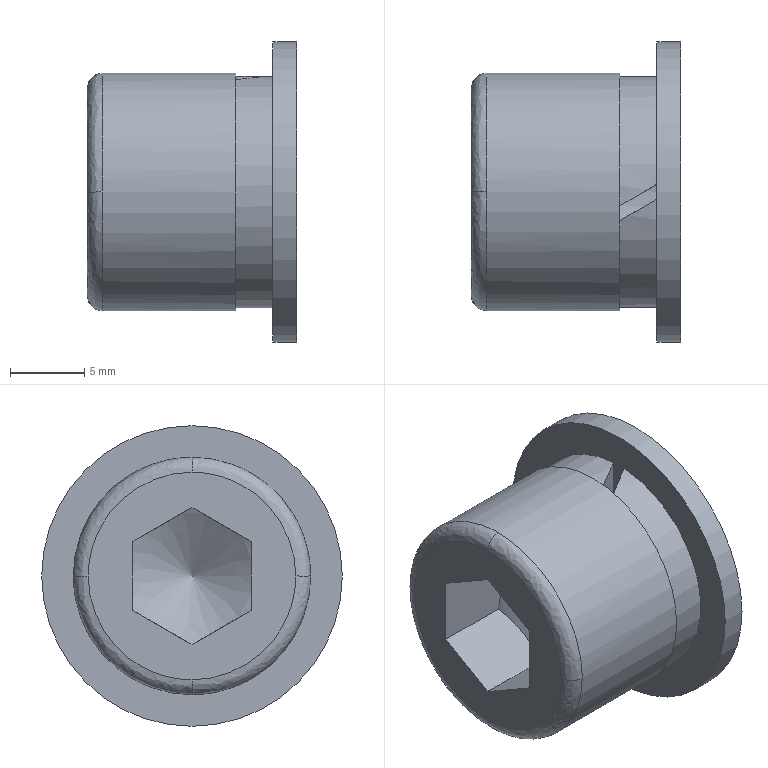Part | NX | features BREP 2 | 2 solids | 23 faces | box 14.1 x 20.25 x 20.25 mm | volume 2295 mm3 | plane 13 | cylinder 5 | spline 4 | cone 1 | commonest cylinder face diameters 10.2 x1 10.7 x1 15.6 x1 16 x1 20.25 x1
STEP:
#1=CARTESIAN_POINT('',(408.903,695.69,-5.1));
#2=VERTEX_POINT('',#1);
#3=CARTESIAN_POINT('',(408.903,695.69,0.));
#4=DIRECTION('',(1.,0.,0.));
#5=DIRECTION('',(0.,0.,-1.));
#6=AXIS2_PLACEMENT_3D('',#3,#4,#5);
#7=CIRCLE('',#6,5.1);
#8=EDGE_CURVE('',#2,#2,#7,.T.);
#9=ORIENTED_EDGE('',*,*,#8,.T.);
#10=EDGE_LOOP('',(#9));
#11=FACE_BOUND('',#10,.T.);
#12=CARTESIAN_POINT('',(408.903,695.69,-10.125));
#13=VERTEX_POINT('',#12);
#14=CARTESIAN_POINT('',(408.903,695.69,0.));
#15=DIRECTION('',(1.,0.,0.));
#16=DIRECTION('',(0.,0.,-1.));
#17=AXIS2_PLACEMENT_3D('',#14,#15,#16);
#18=CIRCLE('',#17,10.125);
#19=EDGE_CURVE('',#13,#13,#18,.T.);
#20=ORIENTED_EDGE('',*,*,#19,.F.);
#21=EDGE_LOOP('',(#20));
#22=FACE_BOUND('',#21,.T.);
#23=CARTESIAN_POINT('',(408.903,705.815,0.));
#24=DIRECTION('',(1.,0.,0.));
#25=DIRECTION('',(0.,0.,1.));
#26=AXIS2_PLACEMENT_3D('',#23,#24,#25);
#27=PLANE('',#26);
#28=ADVANCED_FACE('',(#11,#22),#27,.F.);
#29=CARTESIAN_POINT('',(410.503,695.69,-5.1));
#30=VERTEX_POINT('',#29);
#31=CARTESIAN_POINT('',(410.503,695.69,0.));
#32=DIRECTION('',(1.,0.,0.));
#33=DIRECTION('',(0.,0.,-1.));
#34=AXIS2_PLACEMENT_3D('',#31,#32,#33);
#35=CIRCLE('',#34,5.1);
#36=EDGE_CURVE('',#30,#30,#35,.T.);
#37=ORIENTED_EDGE('',*,*,#36,.F.);
#38=EDGE_LOOP('',(#37));
#39=FACE_BOUND('',#38,.T.);
#40=CARTESIAN_POINT('',(410.503,695.69,-10.125));
#41=VERTEX_POINT('',#40);
#42=CARTESIAN_POINT('',(410.503,695.69,0.));
#43=DIRECTION('',(1.,0.,0.));
#44=DIRECTION('',(0.,0.,-1.));
#45=AXIS2_PLACEMENT_3D('',#42,#43,#44);
#46=CIRCLE('',#45,10.125);
#47=EDGE_CURVE('',#41,#41,#46,.T.);
#48=ORIENTED_EDGE('',*,*,#47,.T.);
#49=EDGE_LOOP('',(#48));
#50=FACE_BOUND('',#49,.T.);
#51=CARTESIAN_POINT('',(410.503,700.79,0.));
#52=DIRECTION('',(1.,0.,0.));
#53=DIRECTION('',(0.,0.,1.));
#54=AXIS2_PLACEMENT_3D('',#51,#52,#53);
#55=PLANE('',#54);
#56=ADVANCED_FACE('',(#39,#50),#55,.T.);
#57=ORIENTED_EDGE('',*,*,#36,.T.);
#58=EDGE_LOOP('',(#57));
#59=FACE_BOUND('',#58,.T.);
#60=ORIENTED_EDGE('',*,*,#8,.F.);
#61=EDGE_LOOP('',(#60));
#62=FACE_BOUND('',#61,.T.);
#63=CARTESIAN_POINT('',(409.703,695.69,0.));
#64=DIRECTION('',(1.,0.,0.));
#65=DIRECTION('',(0.,0.,1.));
#66=AXIS2_PLACEMENT_3D('',#63,#64,#65);
#67=CYLINDRICAL_SURFACE('',#66,5.1);
#68=ADVANCED_FACE('',(#59,#62),#67,.F.);
#69=ORIENTED_EDGE('',*,*,#19,.T.);
#70=EDGE_LOOP('',(#69));
#71=FACE_BOUND('',#70,.T.);
#72=ORIENTED_EDGE('',*,*,#47,.F.);
#73=EDGE_LOOP('',(#72));
#74=FACE_BOUND('',#73,.T.);
#75=CARTESIAN_POINT('',(409.703,695.69,0.));
#76=DIRECTION('',(1.,0.,0.));
#77=DIRECTION('',(0.,0.,1.));
#78=AXIS2_PLACEMENT_3D('',#75,#76,#77);
#79=CYLINDRICAL_SURFACE('',#78,10.125);
#80=ADVANCED_FACE('',(#71,#74),#79,.T.);
#81=CLOSED_SHELL('',(#28,#56,#68,#80));
#82=MANIFOLD_SOLID_BREP('',#81);
#83=CARTESIAN_POINT('',(401.403,691.69,-2.312));
#84=VERTEX_POINT('',#83);
#85=CARTESIAN_POINT('',(401.403,691.69,2.312));
#86=VERTEX_POINT('',#85);
#87=CARTESIAN_POINT('',(401.403,691.69,-2.312));
#88=CARTESIAN_POINT('',(401.622,691.69,-1.557));
#89=CARTESIAN_POINT('',(401.901,691.69,-0.000000056));
#90=CARTESIAN_POINT('',(401.622,691.69,1.557));
#91=CARTESIAN_POINT('',(401.403,691.69,2.312));
#92=B_SPLINE_CURVE_WITH_KNOTS('',3,(#87,#88,#89,#90,#91),.UNSPECIFIED.,.F.,.F.,(4,1,4),(0.,0.002339,0.004679),.UNSPECIFIED.);
#93=EDGE_CURVE('',#84,#86,#92,.T.);
#94=ORIENTED_EDGE('',*,*,#93,.T.);
#95=CARTESIAN_POINT('',(401.403,695.69,4.62));
#96=VERTEX_POINT('',#95);
#97=CARTESIAN_POINT('',(401.403,691.69,2.312));
#98=CARTESIAN_POINT('',(401.621,692.343,2.689));
#99=CARTESIAN_POINT('',(401.9,693.683,3.462));
#100=CARTESIAN_POINT('',(401.621,695.036,4.243));
#101=CARTESIAN_POINT('',(401.403,695.69,4.62));
#102=B_SPLINE_CURVE_WITH_KNOTS('',3,(#97,#98,#99,#100,#101),.UNSPECIFIED.,.F.,.F.,(4,1,4),(0.,0.002332,0.004664),.UNSPECIFIED.);
#103=EDGE_CURVE('',#86,#96,#102,.T.);
#104=ORIENTED_EDGE('',*,*,#103,.T.);
#105=CARTESIAN_POINT('',(401.403,699.69,2.312));
#106=VERTEX_POINT('',#105);
#107=CARTESIAN_POINT('',(401.403,695.69,4.62));
#108=CARTESIAN_POINT('',(401.621,696.343,4.243));
#109=CARTESIAN_POINT('',(401.9,697.683,3.47));
#110=CARTESIAN_POINT('',(401.621,699.036,2.689));
#111=CARTESIAN_POINT('',(401.403,699.69,2.312));
#112=B_SPLINE_CURVE_WITH_KNOTS('',3,(#107,#108,#109,#110,#111),.UNSPECIFIED.,.F.,.F.,(4,1,4),(0.,0.002332,0.004664),.UNSPECIFIED.);
#113=EDGE_CURVE('',#96,#106,#112,.T.);
#114=ORIENTED_EDGE('',*,*,#113,.T.);
#115=CARTESIAN_POINT('',(401.403,699.69,-2.312));
#116=VERTEX_POINT('',#115);
#117=CARTESIAN_POINT('',(401.403,699.69,2.312));
#118=CARTESIAN_POINT('',(401.622,699.69,1.557));
#119=CARTESIAN_POINT('',(401.901,699.69,0.000000056));
#120=CARTESIAN_POINT('',(401.622,699.69,-1.557));
#121=CARTESIAN_POINT('',(401.403,699.69,-2.312));
#122=B_SPLINE_CURVE_WITH_KNOTS('',3,(#117,#118,#119,#120,#121),.UNSPECIFIED.,.F.,.F.,(4,1,4),(0.,0.002339,0.004679),.UNSPECIFIED.);
#123=EDGE_CURVE('',#106,#116,#122,.T.);
#124=ORIENTED_EDGE('',*,*,#123,.T.);
#125=CARTESIAN_POINT('',(401.403,695.69,-4.62));
#126=VERTEX_POINT('',#125);
#127=CARTESIAN_POINT('',(401.403,699.69,-2.312));
#128=CARTESIAN_POINT('',(401.621,699.037,-2.689));
#129=CARTESIAN_POINT('',(401.9,697.698,-3.462));
#130=CARTESIAN_POINT('',(401.621,696.344,-4.243));
#131=CARTESIAN_POINT('',(401.403,695.69,-4.62));
#132=B_SPLINE_CURVE_WITH_KNOTS('',3,(#127,#128,#129,#130,#131),.UNSPECIFIED.,.F.,.F.,(4,1,4),(0.,0.002332,0.004664),.UNSPECIFIED.);
#133=EDGE_CURVE('',#116,#126,#132,.T.);
#134=ORIENTED_EDGE('',*,*,#133,.T.);
#135=CARTESIAN_POINT('',(401.403,695.69,-4.62));
#136=CARTESIAN_POINT('',(401.621,695.037,-4.243));
#137=CARTESIAN_POINT('',(401.9,693.698,-3.47));
#138=CARTESIAN_POINT('',(401.621,692.344,-2.689));
#139=CARTESIAN_POINT('',(401.403,691.69,-2.312));
#140=B_SPLINE_CURVE_WITH_KNOTS('',3,(#135,#136,#137,#138,#139),.UNSPECIFIED.,.F.,.F.,(4,1,4),(0.,0.002332,0.004664),.UNSPECIFIED.);
#141=EDGE_CURVE('',#126,#84,#140,.T.);
#142=ORIENTED_EDGE('',*,*,#141,.T.);
#143=EDGE_LOOP('',(#94,#104,#114,#124,#134,#142));
#144=FACE_BOUND('',#143,.T.);
#145=CARTESIAN_POINT('',(404.071,695.69,0.));
#146=VERTEX_POINT('',#145);
#147=VERTEX_LOOP('',#146);
#148=FACE_BOUND('',#147,.T.);
#149=CARTESIAN_POINT('',(402.737,695.69,0.));
#150=DIRECTION('',(-1.,0.,0.));
#151=DIRECTION('',(0.,-1.,0.));
#152=AXIS2_PLACEMENT_3D('',#149,#150,#151);
#153=CONICAL_SURFACE('',#152,2.31,1.047);
#154=ADVANCED_FACE('',(#144,#148),#153,.F.);
#155=ORIENTED_EDGE('',*,*,#123,.F.);
#156=CARTESIAN_POINT('',(396.403,699.69,2.312));
#157=VERTEX_POINT('',#156);
#158=CARTESIAN_POINT('',(396.403,699.69,2.312));
#159=DIRECTION('',(1.,0.,0.));
#160=VECTOR('',#159,1000.);
#161=LINE('',#158,#160);
#162=EDGE_CURVE('',#157,#106,#161,.T.);
#163=ORIENTED_EDGE('',*,*,#162,.F.);
#164=CARTESIAN_POINT('',(396.403,699.69,-2.312));
#165=VERTEX_POINT('',#164);
#166=CARTESIAN_POINT('',(396.403,699.69,0.));
#167=DIRECTION('',(0.,0.,1.));
#168=VECTOR('',#167,1000.);
#169=LINE('',#166,#168);
#170=EDGE_CURVE('',#165,#157,#169,.T.);
#171=ORIENTED_EDGE('',*,*,#170,.F.);
#172=CARTESIAN_POINT('',(396.403,699.69,-2.312));
#173=DIRECTION('',(1.,0.,0.));
#174=VECTOR('',#173,1000.);
#175=LINE('',#172,#174);
#176=EDGE_CURVE('',#165,#116,#175,.T.);
#177=ORIENTED_EDGE('',*,*,#176,.T.);
#178=EDGE_LOOP('',(#155,#163,#171,#177));
#179=FACE_BOUND('',#178,.T.);
#180=CARTESIAN_POINT('',(396.403,699.69,-2.312));
#181=DIRECTION('',(0.,-1.,0.));
#182=DIRECTION('',(0.,0.,-1.));
#183=AXIS2_PLACEMENT_3D('',#180,#181,#182);
#184=PLANE('',#183);
#185=ADVANCED_FACE('',(#179),#184,.T.);
#186=ORIENTED_EDGE('',*,*,#133,.F.);
#187=ORIENTED_EDGE('',*,*,#176,.F.);
#188=CARTESIAN_POINT('',(396.403,695.69,-4.62));
#189=VERTEX_POINT('',#188);
#190=CARTESIAN_POINT('',(396.403,702.424,-0.7343));
#191=DIRECTION('',(0.,0.8661,0.4998));
#192=VECTOR('',#191,1000.);
#193=LINE('',#190,#192);
#194=EDGE_CURVE('',#189,#165,#193,.T.);
#195=ORIENTED_EDGE('',*,*,#194,.F.);
#196=CARTESIAN_POINT('',(396.403,695.69,-4.62));
#197=DIRECTION('',(-1.,0.,0.));
#198=VECTOR('',#197,1000.);
#199=LINE('',#196,#198);
#200=EDGE_CURVE('',#126,#189,#199,.T.);
#201=ORIENTED_EDGE('',*,*,#200,.F.);
#202=EDGE_LOOP('',(#186,#187,#195,#201));
#203=FACE_BOUND('',#202,.T.);
#204=CARTESIAN_POINT('',(396.403,695.69,-4.62));
#205=DIRECTION('',(0.,-0.4998,0.8661));
#206=DIRECTION('',(1.,0.,0.));
#207=AXIS2_PLACEMENT_3D('',#204,#205,#206);
#208=PLANE('',#207);
#209=ADVANCED_FACE('',(#203),#208,.T.);
#210=ORIENTED_EDGE('',*,*,#141,.F.);
#211=ORIENTED_EDGE('',*,*,#200,.T.);
#212=CARTESIAN_POINT('',(396.403,691.69,-2.312));
#213=VERTEX_POINT('',#212);
#214=CARTESIAN_POINT('',(396.403,698.424,-6.197));
#215=DIRECTION('',(0.,0.8661,-0.4998));
#216=VECTOR('',#215,1000.);
#217=LINE('',#214,#216);
#218=EDGE_CURVE('',#213,#189,#217,.T.);
#219=ORIENTED_EDGE('',*,*,#218,.F.);
#220=CARTESIAN_POINT('',(396.403,691.69,-2.312));
#221=DIRECTION('',(1.,0.,0.));
#222=VECTOR('',#221,1000.);
#223=LINE('',#220,#222);
#224=EDGE_CURVE('',#213,#84,#223,.T.);
#225=ORIENTED_EDGE('',*,*,#224,.T.);
#226=EDGE_LOOP('',(#210,#211,#219,#225));
#227=FACE_BOUND('',#226,.T.);
#228=CARTESIAN_POINT('',(396.403,691.69,-2.312));
#229=DIRECTION('',(0.,0.4998,0.8661));
#230=DIRECTION('',(1.,0.,0.));
#231=AXIS2_PLACEMENT_3D('',#228,#229,#230);
#232=PLANE('',#231);
#233=ADVANCED_FACE('',(#227),#232,.T.);
#234=ORIENTED_EDGE('',*,*,#93,.F.);
#235=ORIENTED_EDGE('',*,*,#224,.F.);
#236=CARTESIAN_POINT('',(396.403,691.69,2.312));
#237=VERTEX_POINT('',#236);
#238=CARTESIAN_POINT('',(396.403,691.69,0.));
#239=DIRECTION('',(0.,0.,-1.));
#240=VECTOR('',#239,1000.);
#241=LINE('',#238,#240);
#242=EDGE_CURVE('',#237,#213,#241,.T.);
#243=ORIENTED_EDGE('',*,*,#242,.F.);
#244=CARTESIAN_POINT('',(396.403,691.69,2.312));
#245=DIRECTION('',(1.,0.,0.));
#246=VECTOR('',#245,1000.);
#247=LINE('',#244,#246);
#248=EDGE_CURVE('',#237,#86,#247,.T.);
#249=ORIENTED_EDGE('',*,*,#248,.T.);
#250=EDGE_LOOP('',(#234,#235,#243,#249));
#251=FACE_BOUND('',#250,.T.);
#252=CARTESIAN_POINT('',(396.403,691.69,2.312));
#253=DIRECTION('',(0.,1.,0.));
#254=DIRECTION('',(0.,0.,1.));
#255=AXIS2_PLACEMENT_3D('',#252,#253,#254);
#256=PLANE('',#255);
#257=ADVANCED_FACE('',(#251),#256,.T.);
#258=ORIENTED_EDGE('',*,*,#103,.F.);
#259=ORIENTED_EDGE('',*,*,#248,.F.);
#260=CARTESIAN_POINT('',(396.403,695.69,4.62));
#261=VERTEX_POINT('',#260);
#262=CARTESIAN_POINT('',(396.403,698.424,6.197));
#263=DIRECTION('',(0.,-0.8661,-0.4998));
#264=VECTOR('',#263,1000.);
#265=LINE('',#262,#264);
#266=EDGE_CURVE('',#261,#237,#265,.T.);
#267=ORIENTED_EDGE('',*,*,#266,.F.);
#268=CARTESIAN_POINT('',(396.403,695.69,4.62));
#269=DIRECTION('',(1.,0.,0.));
#270=VECTOR('',#269,1000.);
#271=LINE('',#268,#270);
#272=EDGE_CURVE('',#261,#96,#271,.T.);
#273=ORIENTED_EDGE('',*,*,#272,.T.);
#274=EDGE_LOOP('',(#258,#259,#267,#273));
#275=FACE_BOUND('',#274,.T.);
#276=CARTESIAN_POINT('',(396.403,695.69,4.62));
#277=DIRECTION('',(0.,0.4998,-0.8661));
#278=DIRECTION('',(-1.,0.,0.));
#279=AXIS2_PLACEMENT_3D('',#276,#277,#278);
#280=PLANE('',#279);
#281=ADVANCED_FACE('',(#275),#280,.T.);
#282=ORIENTED_EDGE('',*,*,#113,.F.);
#283=ORIENTED_EDGE('',*,*,#272,.F.);
#284=CARTESIAN_POINT('',(396.403,702.424,0.7343));
#285=DIRECTION('',(0.,-0.8661,0.4998));
#286=VECTOR('',#285,1000.);
#287=LINE('',#284,#286);
#288=EDGE_CURVE('',#157,#261,#287,.T.);
#289=ORIENTED_EDGE('',*,*,#288,.F.);
#290=ORIENTED_EDGE('',*,*,#162,.T.);
#291=EDGE_LOOP('',(#282,#283,#289,#290));
#292=FACE_BOUND('',#291,.T.);
#293=CARTESIAN_POINT('',(396.403,699.69,2.312));
#294=DIRECTION('',(0.,-0.4998,-0.8661));
#295=DIRECTION('',(-1.,0.,0.));
#296=AXIS2_PLACEMENT_3D('',#293,#294,#295);
#297=PLANE('',#296);
#298=ADVANCED_FACE('',(#292),#297,.T.);
#299=ORIENTED_EDGE('',*,*,#288,.T.);
#300=ORIENTED_EDGE('',*,*,#266,.T.);
#301=ORIENTED_EDGE('',*,*,#242,.T.);
#302=ORIENTED_EDGE('',*,*,#218,.T.);
#303=ORIENTED_EDGE('',*,*,#194,.T.);
#304=ORIENTED_EDGE('',*,*,#170,.T.);
#305=EDGE_LOOP('',(#299,#300,#301,#302,#303,#304));
#306=FACE_BOUND('',#305,.T.);
#307=CARTESIAN_POINT('',(396.403,702.69,0.));
#308=VERTEX_POINT('',#307);
#309=CARTESIAN_POINT('',(396.403,695.69,-7.));
#310=VERTEX_POINT('',#309);
#311=CARTESIAN_POINT('',(396.403,702.69,0.));
#312=CARTESIAN_POINT('',(396.403,702.69,-1.714));
#313=CARTESIAN_POINT('',(396.403,701.233,-5.542));
#314=CARTESIAN_POINT('',(396.403,697.404,-7.));
#315=CARTESIAN_POINT('',(396.403,695.69,-7.));
#316=B_SPLINE_CURVE_WITH_KNOTS('',3,(#311,#312,#313,#314,#315),.UNSPECIFIED.,.F.,.F.,(4,1,4),(0.,8.905,17.809),.UNSPECIFIED.);
#317=EDGE_CURVE('',#308,#310,#316,.T.);
#318=ORIENTED_EDGE('',*,*,#317,.T.);
#319=CARTESIAN_POINT('',(396.403,688.69,0.));
#320=VERTEX_POINT('',#319);
#321=CARTESIAN_POINT('',(396.403,695.69,-7.));
#322=CARTESIAN_POINT('',(396.403,693.977,-7.));
#323=CARTESIAN_POINT('',(396.403,690.148,-5.543));
#324=CARTESIAN_POINT('',(396.403,688.69,-1.714));
#325=CARTESIAN_POINT('',(396.403,688.69,0.));
#326=B_SPLINE_CURVE_WITH_KNOTS('',3,(#321,#322,#323,#324,#325),.UNSPECIFIED.,.F.,.F.,(4,1,4),(0.,8.905,17.809),.UNSPECIFIED.);
#327=EDGE_CURVE('',#310,#320,#326,.T.);
#328=ORIENTED_EDGE('',*,*,#327,.T.);
#329=CARTESIAN_POINT('',(396.403,695.69,7.));
#330=VERTEX_POINT('',#329);
#331=CARTESIAN_POINT('',(396.403,688.69,0.));
#332=CARTESIAN_POINT('',(396.403,688.69,1.714));
#333=CARTESIAN_POINT('',(396.403,690.147,5.542));
#334=CARTESIAN_POINT('',(396.403,693.977,7.));
#335=CARTESIAN_POINT('',(396.403,695.69,7.));
#336=B_SPLINE_CURVE_WITH_KNOTS('',3,(#331,#332,#333,#334,#335),.UNSPECIFIED.,.F.,.F.,(4,1,4),(0.,8.905,17.809),.UNSPECIFIED.);
#337=EDGE_CURVE('',#320,#330,#336,.T.);
#338=ORIENTED_EDGE('',*,*,#337,.T.);
#339=CARTESIAN_POINT('',(396.403,695.69,7.));
#340=CARTESIAN_POINT('',(396.403,697.404,7.));
#341=CARTESIAN_POINT('',(396.403,701.233,5.543));
#342=CARTESIAN_POINT('',(396.403,702.69,1.714));
#343=CARTESIAN_POINT('',(396.403,702.69,0.));
#344=B_SPLINE_CURVE_WITH_KNOTS('',3,(#339,#340,#341,#342,#343),.UNSPECIFIED.,.F.,.F.,(4,1,4),(0.,8.905,17.809),.UNSPECIFIED.);
#345=EDGE_CURVE('',#330,#308,#344,.T.);
#346=ORIENTED_EDGE('',*,*,#345,.T.);
#347=EDGE_LOOP('',(#318,#328,#338,#346));
#348=FACE_BOUND('',#347,.T.);
#349=CARTESIAN_POINT('',(396.403,702.,0.));
#350=DIRECTION('',(-1.,0.,0.));
#351=DIRECTION('',(0.,0.,1.));
#352=AXIS2_PLACEMENT_3D('',#349,#350,#351);
#353=PLANE('',#352);
#354=ADVANCED_FACE('',(#306,#348),#353,.T.);
#355=CARTESIAN_POINT('',(397.403,687.69,0.));
#356=VERTEX_POINT('',#355);
#357=CARTESIAN_POINT('',(397.403,695.69,8.));
#358=VERTEX_POINT('',#357);
#359=CARTESIAN_POINT('',(397.403,695.69,8.));
#360=CARTESIAN_POINT('',(397.403,693.596,8.));
#361=CARTESIAN_POINT('',(397.403,689.424,6.267));
#362=CARTESIAN_POINT('',(397.403,687.69,2.094));
#363=CARTESIAN_POINT('',(397.403,687.69,0.));
#364=B_SPLINE_CURVE_WITH_KNOTS('',3,(#359,#360,#361,#362,#363),.UNSPECIFIED.,.F.,.F.,(4,1,4),(0.,0.5,1.),.UNSPECIFIED.);
#365=EDGE_CURVE('',#356,#358,#364,.F.);
#366=ORIENTED_EDGE('',*,*,#365,.T.);
#367=CARTESIAN_POINT('',(397.403,695.69,8.));
#368=CARTESIAN_POINT('',(397.168,695.69,8.));
#369=CARTESIAN_POINT('',(396.607,695.69,7.796));
#370=CARTESIAN_POINT('',(396.403,695.69,7.236));
#371=CARTESIAN_POINT('',(396.403,695.69,7.));
#372=B_SPLINE_CURVE_WITH_KNOTS('',3,(#367,#368,#369,#370,#371),.UNSPECIFIED.,.F.,.F.,(4,1,4),(0.,1.069,2.138),.UNSPECIFIED.);
#373=EDGE_CURVE('',#358,#330,#372,.T.);
#374=ORIENTED_EDGE('',*,*,#373,.T.);
#375=ORIENTED_EDGE('',*,*,#337,.F.);
#376=CARTESIAN_POINT('',(396.403,688.69,0.));
#377=CARTESIAN_POINT('',(396.403,688.455,0.));
#378=CARTESIAN_POINT('',(396.607,687.894,0.));
#379=CARTESIAN_POINT('',(397.168,687.69,0.));
#380=CARTESIAN_POINT('',(397.403,687.69,0.));
#381=B_SPLINE_CURVE_WITH_KNOTS('',3,(#376,#377,#378,#379,#380),.UNSPECIFIED.,.F.,.F.,(4,1,4),(0.,1.069,2.138),.UNSPECIFIED.);
#382=EDGE_CURVE('',#356,#320,#381,.F.);
#383=ORIENTED_EDGE('',*,*,#382,.F.);
#384=EDGE_LOOP('',(#366,#374,#375,#383));
#385=FACE_BOUND('',#384,.T.);
#386=CARTESIAN_POINT('',(397.403,687.69,0.));
#387=CARTESIAN_POINT('',(397.403,687.69,8.));
#388=CARTESIAN_POINT('',(397.403,695.69,8.));
#389=CARTESIAN_POINT('',(396.403,687.69,0.));
#390=CARTESIAN_POINT('',(396.403,687.69,8.));
#391=CARTESIAN_POINT('',(396.403,695.69,8.));
#392=CARTESIAN_POINT('',(396.403,688.69,0.));
#393=CARTESIAN_POINT('',(396.403,688.69,7.));
#394=CARTESIAN_POINT('',(396.403,695.69,7.));
#395=(BOUNDED_SURFACE()B_SPLINE_SURFACE(2,2,((#386,#387,#388),(#389,#390,#391),(#392,#393,#394)),.TOROIDAL_SURF.,.F.,.F.,.F.)B_SPLINE_SURFACE_WITH_KNOTS((3,3),(3,3),(0.,2.138),(14.,29.333),.PIECEWISE_BEZIER_KNOTS.)GEOMETRIC_REPRESENTATION_ITEM()RATIONAL_B_SPLINE_SURFACE(((1.,0.7071,1.),(0.7071,0.5,0.7071),(1.,0.7071,1.)))REPRESENTATION_ITEM('')SURFACE());
#396=ADVANCED_FACE('',(#385),#395,.F.);
#397=ORIENTED_EDGE('',*,*,#345,.F.);
#398=ORIENTED_EDGE('',*,*,#373,.F.);
#399=CARTESIAN_POINT('',(397.403,703.69,0.));
#400=VERTEX_POINT('',#399);
#401=CARTESIAN_POINT('',(397.403,703.69,0.));
#402=CARTESIAN_POINT('',(397.403,703.69,2.094));
#403=CARTESIAN_POINT('',(397.403,701.957,6.267));
#404=CARTESIAN_POINT('',(397.403,697.785,8.));
#405=CARTESIAN_POINT('',(397.403,695.69,8.));
#406=B_SPLINE_CURVE_WITH_KNOTS('',3,(#401,#402,#403,#404,#405),.UNSPECIFIED.,.F.,.F.,(4,1,4),(0.,0.5,1.),.UNSPECIFIED.);
#407=EDGE_CURVE('',#358,#400,#406,.F.);
#408=ORIENTED_EDGE('',*,*,#407,.T.);
#409=CARTESIAN_POINT('',(397.403,703.69,0.));
#410=CARTESIAN_POINT('',(397.168,703.69,0.));
#411=CARTESIAN_POINT('',(396.607,703.487,0.));
#412=CARTESIAN_POINT('',(396.403,702.926,0.));
#413=CARTESIAN_POINT('',(396.403,702.69,0.));
#414=B_SPLINE_CURVE_WITH_KNOTS('',3,(#409,#410,#411,#412,#413),.UNSPECIFIED.,.F.,.F.,(4,1,4),(0.,1.069,2.138),.UNSPECIFIED.);
#415=EDGE_CURVE('',#400,#308,#414,.T.);
#416=ORIENTED_EDGE('',*,*,#415,.T.);
#417=EDGE_LOOP('',(#397,#398,#408,#416));
#418=FACE_BOUND('',#417,.T.);
#419=CARTESIAN_POINT('',(397.403,695.69,8.));
#420=CARTESIAN_POINT('',(397.403,703.69,8.));
#421=CARTESIAN_POINT('',(397.403,703.69,0.));
#422=CARTESIAN_POINT('',(396.403,695.69,8.));
#423=CARTESIAN_POINT('',(396.403,703.69,8.));
#424=CARTESIAN_POINT('',(396.403,703.69,0.));
#425=CARTESIAN_POINT('',(396.403,695.69,7.));
#426=CARTESIAN_POINT('',(396.403,702.69,7.));
#427=CARTESIAN_POINT('',(396.403,702.69,0.));
#428=(BOUNDED_SURFACE()B_SPLINE_SURFACE(2,2,((#419,#420,#421),(#422,#423,#424),(#425,#426,#427)),.TOROIDAL_SURF.,.F.,.F.,.F.)B_SPLINE_SURFACE_WITH_KNOTS((3,3),(3,3),(0.,2.138),(28.,43.333),.PIECEWISE_BEZIER_KNOTS.)GEOMETRIC_REPRESENTATION_ITEM()RATIONAL_B_SPLINE_SURFACE(((1.,0.7071,1.),(0.7071,0.5,0.7071),(1.,0.7071,1.)))REPRESENTATION_ITEM('')SURFACE());
#429=ADVANCED_FACE('',(#418),#428,.F.);
#430=CARTESIAN_POINT('',(397.403,695.69,-8.));
#431=VERTEX_POINT('',#430);
#432=CARTESIAN_POINT('',(397.403,695.69,-8.));
#433=CARTESIAN_POINT('',(397.403,697.785,-8.));
#434=CARTESIAN_POINT('',(397.403,701.957,-6.267));
#435=CARTESIAN_POINT('',(397.403,703.69,-2.094));
#436=CARTESIAN_POINT('',(397.403,703.69,0.));
#437=B_SPLINE_CURVE_WITH_KNOTS('',3,(#432,#433,#434,#435,#436),.UNSPECIFIED.,.F.,.F.,(4,1,4),(0.,0.5,1.),.UNSPECIFIED.);
#438=EDGE_CURVE('',#400,#431,#437,.F.);
#439=ORIENTED_EDGE('',*,*,#438,.T.);
#440=CARTESIAN_POINT('',(397.403,695.69,-8.));
#441=CARTESIAN_POINT('',(397.168,695.69,-8.));
#442=CARTESIAN_POINT('',(396.607,695.69,-7.796));
#443=CARTESIAN_POINT('',(396.403,695.69,-7.236));
#444=CARTESIAN_POINT('',(396.403,695.69,-7.));
#445=B_SPLINE_CURVE_WITH_KNOTS('',3,(#440,#441,#442,#443,#444),.UNSPECIFIED.,.F.,.F.,(4,1,4),(0.,1.069,2.138),.UNSPECIFIED.);
#446=EDGE_CURVE('',#431,#310,#445,.T.);
#447=ORIENTED_EDGE('',*,*,#446,.T.);
#448=ORIENTED_EDGE('',*,*,#317,.F.);
#449=ORIENTED_EDGE('',*,*,#415,.F.);
#450=EDGE_LOOP('',(#439,#447,#448,#449));
#451=FACE_BOUND('',#450,.T.);
#452=CARTESIAN_POINT('',(397.403,703.69,0.));
#453=CARTESIAN_POINT('',(397.403,703.69,-8.));
#454=CARTESIAN_POINT('',(397.403,695.69,-8.));
#455=CARTESIAN_POINT('',(396.403,703.69,0.));
#456=CARTESIAN_POINT('',(396.403,703.69,-8.));
#457=CARTESIAN_POINT('',(396.403,695.69,-8.));
#458=CARTESIAN_POINT('',(396.403,702.69,0.));
#459=CARTESIAN_POINT('',(396.403,702.69,-7.));
#460=CARTESIAN_POINT('',(396.403,695.69,-7.));
#461=(BOUNDED_SURFACE()B_SPLINE_SURFACE(2,2,((#452,#453,#454),(#455,#456,#457),(#458,#459,#460)),.TOROIDAL_SURF.,.F.,.F.,.F.)B_SPLINE_SURFACE_WITH_KNOTS((3,3),(3,3),(0.,2.138),(42.,57.333),.PIECEWISE_BEZIER_KNOTS.)GEOMETRIC_REPRESENTATION_ITEM()RATIONAL_B_SPLINE_SURFACE(((1.,0.7071,1.),(0.7071,0.5,0.7071),(1.,0.7071,1.)))REPRESENTATION_ITEM('')SURFACE());
#462=ADVANCED_FACE('',(#451),#461,.F.);
#463=ORIENTED_EDGE('',*,*,#327,.F.);
#464=ORIENTED_EDGE('',*,*,#446,.F.);
#465=CARTESIAN_POINT('',(397.403,687.69,0.));
#466=CARTESIAN_POINT('',(397.403,687.69,-2.094));
#467=CARTESIAN_POINT('',(397.403,689.424,-6.267));
#468=CARTESIAN_POINT('',(397.403,693.596,-8.));
#469=CARTESIAN_POINT('',(397.403,695.69,-8.));
#470=B_SPLINE_CURVE_WITH_KNOTS('',3,(#465,#466,#467,#468,#469),.UNSPECIFIED.,.F.,.F.,(4,1,4),(0.,0.5,1.),.UNSPECIFIED.);
#471=EDGE_CURVE('',#431,#356,#470,.F.);
#472=ORIENTED_EDGE('',*,*,#471,.T.);
#473=ORIENTED_EDGE('',*,*,#382,.T.);
#474=EDGE_LOOP('',(#463,#464,#472,#473));
#475=FACE_BOUND('',#474,.T.);
#476=CARTESIAN_POINT('',(397.403,695.69,-8.));
#477=CARTESIAN_POINT('',(397.403,687.69,-8.));
#478=CARTESIAN_POINT('',(397.403,687.69,0.));
#479=CARTESIAN_POINT('',(396.403,695.69,-8.));
#480=CARTESIAN_POINT('',(396.403,687.69,-8.));
#481=CARTESIAN_POINT('',(396.403,687.69,0.));
#482=CARTESIAN_POINT('',(396.403,695.69,-7.));
#483=CARTESIAN_POINT('',(396.403,688.69,-7.));
#484=CARTESIAN_POINT('',(396.403,688.69,0.));
#485=(BOUNDED_SURFACE()B_SPLINE_SURFACE(2,2,((#476,#477,#478),(#479,#480,#481),(#482,#483,#484)),.TOROIDAL_SURF.,.F.,.F.,.F.)B_SPLINE_SURFACE_WITH_KNOTS((3,3),(3,3),(0.,2.138),(0.,15.333),.PIECEWISE_BEZIER_KNOTS.)GEOMETRIC_REPRESENTATION_ITEM()RATIONAL_B_SPLINE_SURFACE(((1.,0.7071,1.),(0.7071,0.5,0.7071),(1.,0.7071,1.)))REPRESENTATION_ITEM('')SURFACE());
#486=ADVANCED_FACE('',(#475),#485,.F.);
#487=CARTESIAN_POINT('',(406.403,693.747,7.554));
#488=VERTEX_POINT('',#487);
#489=CARTESIAN_POINT('',(406.403,693.747,4.985));
#490=VERTEX_POINT('',#489);
#491=CARTESIAN_POINT('',(406.403,693.747,0.));
#492=DIRECTION('',(0.,0.,-1.));
#493=VECTOR('',#492,1000.);
#494=LINE('',#491,#493);
#495=EDGE_CURVE('',#488,#490,#494,.T.);
#496=ORIENTED_EDGE('',*,*,#495,.F.);
#497=CARTESIAN_POINT('',(408.903,695.19,7.784));
#498=VERTEX_POINT('',#497);
#499=CARTESIAN_POINT('',(409.769,695.69,0.));
#500=DIRECTION('',(0.5,-0.866,0.));
#501=DIRECTION('',(0.866,0.5,0.));
#502=AXIS2_PLACEMENT_3D('',#499,#500,#501);
#503=ELLIPSE('',#502,15.6,7.8);
#504=EDGE_CURVE('',#498,#488,#503,.T.);
#505=ORIENTED_EDGE('',*,*,#504,.F.);
#506=CARTESIAN_POINT('',(408.903,695.19,5.327));
#507=VERTEX_POINT('',#506);
#508=CARTESIAN_POINT('',(408.903,695.19,0.));
#509=DIRECTION('',(0.,0.,-1.));
#510=VECTOR('',#509,1000.);
#511=LINE('',#508,#510);
#512=EDGE_CURVE('',#498,#507,#511,.T.);
#513=ORIENTED_EDGE('',*,*,#512,.T.);
#514=CARTESIAN_POINT('',(409.769,695.69,0.));
#515=DIRECTION('',(0.5,-0.866,0.));
#516=DIRECTION('',(0.866,0.5,0.));
#517=AXIS2_PLACEMENT_3D('',#514,#515,#516);
#518=ELLIPSE('',#517,10.7,5.35);
#519=EDGE_CURVE('',#490,#507,#518,.F.);
#520=ORIENTED_EDGE('',*,*,#519,.F.);
#521=EDGE_LOOP('',(#496,#505,#513,#520));
#522=FACE_BOUND('',#521,.T.);
#523=CARTESIAN_POINT('',(408.903,695.19,0.));
#524=DIRECTION('',(0.5,-0.866,0.));
#525=DIRECTION('',(0.,0.,-1.));
#526=AXIS2_PLACEMENT_3D('',#523,#524,#525);
#527=PLANE('',#526);
#528=ADVANCED_FACE('',(#522),#527,.F.);
#529=CARTESIAN_POINT('',(406.403,694.747,7.743));
#530=VERTEX_POINT('',#529);
#531=CARTESIAN_POINT('',(406.403,695.69,0.));
#532=DIRECTION('',(1.,0.,0.));
#533=DIRECTION('',(0.,0.,-1.));
#534=AXIS2_PLACEMENT_3D('',#531,#532,#533);
#535=CIRCLE('',#534,7.8);
#536=EDGE_CURVE('',#488,#530,#535,.T.);
#537=ORIENTED_EDGE('',*,*,#536,.T.);
#538=CARTESIAN_POINT('',(408.903,696.19,7.784));
#539=VERTEX_POINT('',#538);
#540=CARTESIAN_POINT('',(408.037,695.69,0.));
#541=DIRECTION('',(-0.5,0.866,0.));
#542=DIRECTION('',(0.866,0.5,0.));
#543=AXIS2_PLACEMENT_3D('',#540,#541,#542);
#544=ELLIPSE('',#543,15.6,7.8);
#545=EDGE_CURVE('',#539,#530,#544,.F.);
#546=ORIENTED_EDGE('',*,*,#545,.F.);
#547=CARTESIAN_POINT('',(408.903,695.69,0.));
#548=DIRECTION('',(1.,0.,0.));
#549=DIRECTION('',(0.,0.,-1.));
#550=AXIS2_PLACEMENT_3D('',#547,#548,#549);
#551=CIRCLE('',#550,7.8);
#552=EDGE_CURVE('',#539,#498,#551,.F.);
#553=ORIENTED_EDGE('',*,*,#552,.T.);
#554=ORIENTED_EDGE('',*,*,#504,.T.);
#555=EDGE_LOOP('',(#537,#546,#553,#554));
#556=FACE_BOUND('',#555,.T.);
#557=CARTESIAN_POINT('',(407.653,695.69,0.));
#558=DIRECTION('',(1.,0.,0.));
#559=DIRECTION('',(0.,0.,1.));
#560=AXIS2_PLACEMENT_3D('',#557,#558,#559);
#561=CYLINDRICAL_SURFACE('',#560,7.8);
#562=ADVANCED_FACE('',(#556),#561,.T.);
#563=ORIENTED_EDGE('',*,*,#438,.F.);
#564=ORIENTED_EDGE('',*,*,#407,.F.);
#565=ORIENTED_EDGE('',*,*,#365,.F.);
#566=ORIENTED_EDGE('',*,*,#471,.F.);
#567=EDGE_LOOP('',(#563,#564,#565,#566));
#568=FACE_BOUND('',#567,.T.);
#569=CARTESIAN_POINT('',(406.403,695.69,-8.));
#570=VERTEX_POINT('',#569);
#571=CARTESIAN_POINT('',(406.403,695.69,0.));
#572=DIRECTION('',(1.,0.,0.));
#573=DIRECTION('',(0.,0.,-1.));
#574=AXIS2_PLACEMENT_3D('',#571,#572,#573);
#575=CIRCLE('',#574,8.);
#576=EDGE_CURVE('',#570,#570,#575,.F.);
#577=ORIENTED_EDGE('',*,*,#576,.T.);
#578=EDGE_LOOP('',(#577));
#579=FACE_BOUND('',#578,.T.);
#580=CARTESIAN_POINT('',(401.403,695.69,0.));
#581=DIRECTION('',(-1.,0.,0.));
#582=DIRECTION('',(0.,-1.,0.));
#583=AXIS2_PLACEMENT_3D('',#580,#581,#582);
#584=CYLINDRICAL_SURFACE('',#583,8.);
#585=ADVANCED_FACE('',(#568,#579),#584,.T.);
#586=CARTESIAN_POINT('',(406.403,694.747,5.266));
#587=VERTEX_POINT('',#586);
#588=CARTESIAN_POINT('',(406.403,694.747,0.));
#589=DIRECTION('',(0.,0.,1.));
#590=VECTOR('',#589,1000.);
#591=LINE('',#588,#590);
#592=EDGE_CURVE('',#587,#530,#591,.T.);
#593=ORIENTED_EDGE('',*,*,#592,.F.);
#594=CARTESIAN_POINT('',(408.903,696.19,5.327));
#595=VERTEX_POINT('',#594);
#596=CARTESIAN_POINT('',(408.037,695.69,0.));
#597=DIRECTION('',(-0.5,0.866,0.));
#598=DIRECTION('',(0.866,0.5,0.));
#599=AXIS2_PLACEMENT_3D('',#596,#597,#598);
#600=ELLIPSE('',#599,10.7,5.35);
#601=EDGE_CURVE('',#595,#587,#600,.F.);
#602=ORIENTED_EDGE('',*,*,#601,.F.);
#603=CARTESIAN_POINT('',(408.903,696.19,0.));
#604=DIRECTION('',(0.,0.,-1.));
#605=VECTOR('',#604,1000.);
#606=LINE('',#603,#605);
#607=EDGE_CURVE('',#539,#595,#606,.T.);
#608=ORIENTED_EDGE('',*,*,#607,.F.);
#609=ORIENTED_EDGE('',*,*,#545,.T.);
#610=EDGE_LOOP('',(#593,#602,#608,#609));
#611=FACE_BOUND('',#610,.T.);
#612=CARTESIAN_POINT('',(406.403,694.747,0.));
#613=DIRECTION('',(-0.5,0.866,0.));
#614=DIRECTION('',(0.,0.,1.));
#615=AXIS2_PLACEMENT_3D('',#612,#613,#614);
#616=PLANE('',#615);
#617=ADVANCED_FACE('',(#611),#616,.F.);
#618=ORIENTED_EDGE('',*,*,#607,.T.);
#619=CARTESIAN_POINT('',(408.903,695.69,0.));
#620=DIRECTION('',(1.,0.,0.));
#621=DIRECTION('',(0.,0.,-1.));
#622=AXIS2_PLACEMENT_3D('',#619,#620,#621);
#623=CIRCLE('',#622,5.35);
#624=EDGE_CURVE('',#507,#595,#623,.T.);
#625=ORIENTED_EDGE('',*,*,#624,.F.);
#626=ORIENTED_EDGE('',*,*,#512,.F.);
#627=ORIENTED_EDGE('',*,*,#552,.F.);
#628=EDGE_LOOP('',(#618,#625,#626,#627));
#629=FACE_BOUND('',#628,.T.);
#630=CARTESIAN_POINT('',(408.903,702.365,0.));
#631=DIRECTION('',(1.,0.,0.));
#632=DIRECTION('',(0.,0.,-1.));
#633=AXIS2_PLACEMENT_3D('',#630,#631,#632);
#634=PLANE('',#633);
#635=ADVANCED_FACE('',(#629),#634,.T.);
#636=ORIENTED_EDGE('',*,*,#592,.T.);
#637=ORIENTED_EDGE('',*,*,#536,.F.);
#638=ORIENTED_EDGE('',*,*,#495,.T.);
#639=CARTESIAN_POINT('',(406.403,695.69,0.));
#640=DIRECTION('',(1.,0.,0.));
#641=DIRECTION('',(0.,0.,-1.));
#642=AXIS2_PLACEMENT_3D('',#639,#640,#641);
#643=CIRCLE('',#642,5.35);
#644=EDGE_CURVE('',#490,#587,#643,.T.);
#645=ORIENTED_EDGE('',*,*,#644,.T.);
#646=EDGE_LOOP('',(#636,#637,#638,#645));
#647=FACE_BOUND('',#646,.T.);
#648=ORIENTED_EDGE('',*,*,#576,.F.);
#649=EDGE_LOOP('',(#648));
#650=FACE_BOUND('',#649,.T.);
#651=CARTESIAN_POINT('',(406.403,695.69,0.));
#652=DIRECTION('',(1.,0.,0.));
#653=DIRECTION('',(0.,1.,0.));
#654=AXIS2_PLACEMENT_3D('',#651,#652,#653);
#655=PLANE('',#654);
#656=ADVANCED_FACE('',(#647,#650),#655,.T.);
#657=ORIENTED_EDGE('',*,*,#624,.T.);
#658=ORIENTED_EDGE('',*,*,#601,.T.);
#659=ORIENTED_EDGE('',*,*,#644,.F.);
#660=ORIENTED_EDGE('',*,*,#519,.T.);
#661=EDGE_LOOP('',(#657,#658,#659,#660));
#662=FACE_BOUND('',#661,.T.);
#663=CARTESIAN_POINT('',(407.653,695.69,0.));
#664=DIRECTION('',(1.,0.,0.));
#665=DIRECTION('',(0.,1.,0.));
#666=AXIS2_PLACEMENT_3D('',#663,#664,#665);
#667=CYLINDRICAL_SURFACE('',#666,5.35);
#668=ADVANCED_FACE('',(#662),#667,.F.);
#669=CLOSED_SHELL('',(#154,#185,#209,#233,#257,#281,#298,#354,#396,#429,#462,#486,#528,#562,#585,#617,#635,#656,#668));
#670=MANIFOLD_SOLID_BREP('',#669);
#671=(LENGTH_UNIT()NAMED_UNIT(*)SI_UNIT(.MILLI.,.METRE.));
#672=UNCERTAINTY_MEASURE_WITH_UNIT(LENGTH_MEASURE(0.0508),#671,'','');
#673=(NAMED_UNIT(*)PLANE_ANGLE_UNIT()SI_UNIT($,.RADIAN.));
#674=(NAMED_UNIT(*)SI_UNIT($,.STERADIAN.)SOLID_ANGLE_UNIT());
#675=(GEOMETRIC_REPRESENTATION_CONTEXT(3)GLOBAL_UNCERTAINTY_ASSIGNED_CONTEXT((#672))GLOBAL_UNIT_ASSIGNED_CONTEXT((#671,#673,#674))REPRESENTATION_CONTEXT('',''));
#676=ADVANCED_BREP_SHAPE_REPRESENTATION('',(#82,#670),#675);